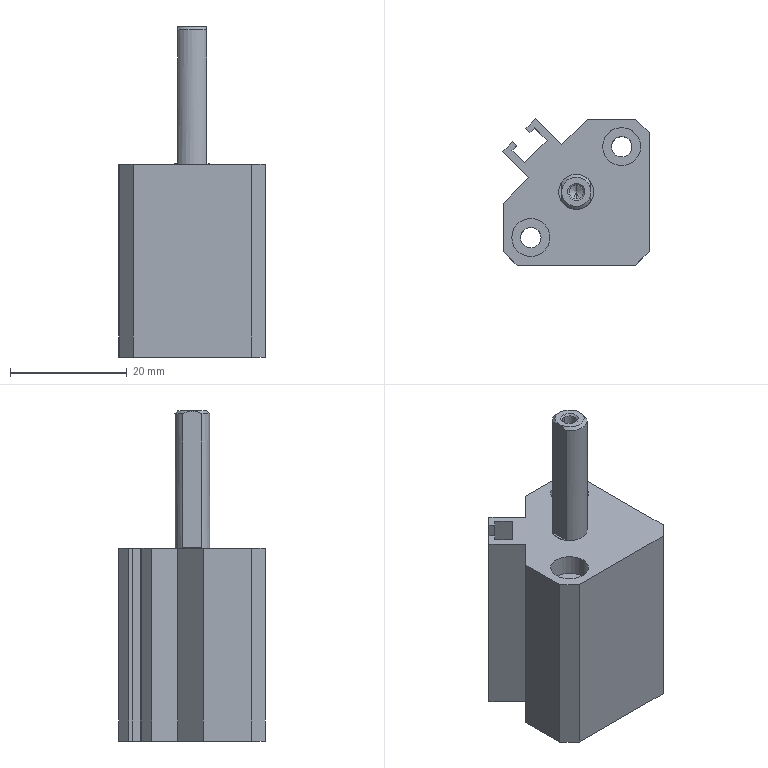Part | STEP file | ASND-0110-CDQ2B12-5D(0)aq | 1 solid | 63 faces | box 25.087 x 25.087 x 56.5 mm | volume 17303 mm3 | plane 33 | cylinder 20 | cone 10 | commonest cylinder face diameters 6.5 x8 3.5 x4 4.13 x4 2.39 x2 6 x2